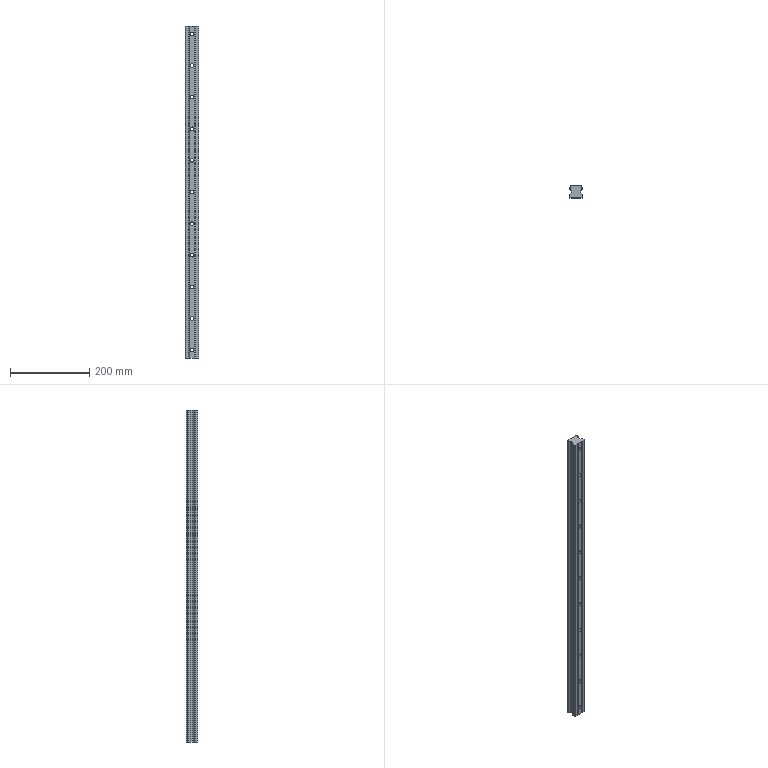Part | STEP file | Slide Rail HGR35R840C | 1 solid | 95 faces | box 34 x 29 x 840 mm | volume 682718 mm3 | cylinder 54 | plane 41 | commonest cylinder face diameters 9 x22 14 x22 2.4 x6 6.5 x4